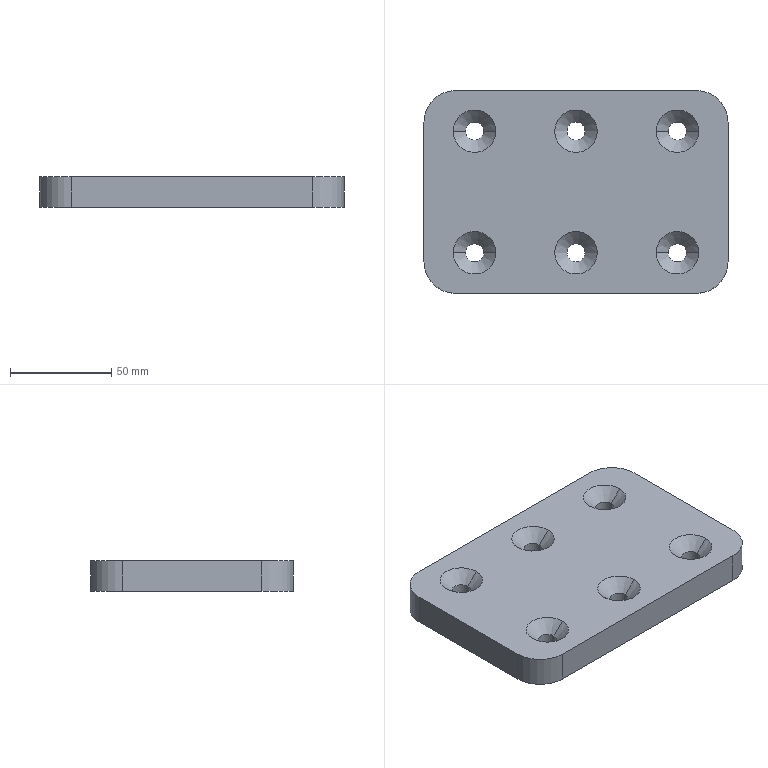Part | SolidWorks | features BaseBody 1 | 1 solid | 48 faces | box 150 x 100 x 15 mm | volume 211756 mm3 | plane 20 | cylinder 16 | cone 12 | commonest cylinder face diameters 9 x12 31 x4
STEP:
#1=CARTESIAN_POINT('',(-50.5,310.,-51.));
#2=VERTEX_POINT('',#1);
#3=CARTESIAN_POINT('',(-41.5,310.,-51.));
#4=VERTEX_POINT('',#3);
#5=CARTESIAN_POINT('',(-46.,310.,-51.));
#6=DIRECTION('',(0.,0.,-1.));
#7=DIRECTION('',(-1.,0.,0.));
#8=AXIS2_PLACEMENT_3D('',#5,#6,#7);
#9=CIRCLE('',#8,4.5);
#10=EDGE_CURVE('',#2,#4,#9,.T.);
#11=ORIENTED_EDGE('',*,*,#10,.F.);
#12=CARTESIAN_POINT('',(-50.5,310.,-60.));
#13=VERTEX_POINT('',#12);
#14=CARTESIAN_POINT('',(-50.5,310.,-40.));
#15=DIRECTION('',(0.,0.,-1.));
#16=VECTOR('',#15,1000.);
#17=LINE('',#14,#16);
#18=EDGE_CURVE('',#2,#13,#17,.T.);
#19=ORIENTED_EDGE('',*,*,#18,.T.);
#20=CARTESIAN_POINT('',(-41.5,310.,-60.));
#21=VERTEX_POINT('',#20);
#22=CARTESIAN_POINT('',(-46.,310.,-60.));
#23=DIRECTION('',(0.,0.,-1.));
#24=DIRECTION('',(1.,0.,0.));
#25=AXIS2_PLACEMENT_3D('',#22,#23,#24);
#26=CIRCLE('',#25,4.5);
#27=EDGE_CURVE('',#13,#21,#26,.T.);
#28=ORIENTED_EDGE('',*,*,#27,.T.);
#29=CARTESIAN_POINT('',(-41.5,310.,-40.));
#30=DIRECTION('',(0.,0.,-1.));
#31=VECTOR('',#30,1000.);
#32=LINE('',#29,#31);
#33=EDGE_CURVE('',#4,#21,#32,.T.);
#34=ORIENTED_EDGE('',*,*,#33,.F.);
#35=EDGE_LOOP('',(#11,#19,#28,#34));
#36=FACE_OUTER_BOUND('',#35,.T.);
#37=CARTESIAN_POINT('',(-46.,310.,-40.));
#38=DIRECTION('',(0.,0.,-1.));
#39=DIRECTION('',(1.,0.,0.));
#40=AXIS2_PLACEMENT_3D('',#37,#38,#39);
#41=CYLINDRICAL_SURFACE('',#40,4.5);
#42=ADVANCED_FACE('',(#36),#41,.F.);
#43=CARTESIAN_POINT('',(-50.5,250.,-51.));
#44=VERTEX_POINT('',#43);
#45=CARTESIAN_POINT('',(-41.5,250.,-51.));
#46=VERTEX_POINT('',#45);
#47=CARTESIAN_POINT('',(-46.,250.,-51.));
#48=DIRECTION('',(0.,0.,-1.));
#49=DIRECTION('',(-1.,0.,0.));
#50=AXIS2_PLACEMENT_3D('',#47,#48,#49);
#51=CIRCLE('',#50,4.5);
#52=EDGE_CURVE('',#44,#46,#51,.T.);
#53=ORIENTED_EDGE('',*,*,#52,.F.);
#54=CARTESIAN_POINT('',(-50.5,250.,-60.));
#55=VERTEX_POINT('',#54);
#56=CARTESIAN_POINT('',(-50.5,250.,-40.));
#57=DIRECTION('',(0.,0.,-1.));
#58=VECTOR('',#57,1000.);
#59=LINE('',#56,#58);
#60=EDGE_CURVE('',#44,#55,#59,.T.);
#61=ORIENTED_EDGE('',*,*,#60,.T.);
#62=CARTESIAN_POINT('',(-41.5,250.,-60.));
#63=VERTEX_POINT('',#62);
#64=CARTESIAN_POINT('',(-46.,250.,-60.));
#65=DIRECTION('',(0.,0.,-1.));
#66=DIRECTION('',(1.,0.,0.));
#67=AXIS2_PLACEMENT_3D('',#64,#65,#66);
#68=CIRCLE('',#67,4.5);
#69=EDGE_CURVE('',#55,#63,#68,.T.);
#70=ORIENTED_EDGE('',*,*,#69,.T.);
#71=CARTESIAN_POINT('',(-41.5,250.,-40.));
#72=DIRECTION('',(0.,0.,-1.));
#73=VECTOR('',#72,1000.);
#74=LINE('',#71,#73);
#75=EDGE_CURVE('',#46,#63,#74,.T.);
#76=ORIENTED_EDGE('',*,*,#75,.F.);
#77=EDGE_LOOP('',(#53,#61,#70,#76));
#78=FACE_OUTER_BOUND('',#77,.T.);
#79=CARTESIAN_POINT('',(-46.,250.,-40.));
#80=DIRECTION('',(0.,0.,-1.));
#81=DIRECTION('',(1.,0.,0.));
#82=AXIS2_PLACEMENT_3D('',#79,#80,#81);
#83=CYLINDRICAL_SURFACE('',#82,4.5);
#84=ADVANCED_FACE('',(#78),#83,.F.);
#85=CARTESIAN_POINT('',(-100.5,310.,-51.));
#86=VERTEX_POINT('',#85);
#87=CARTESIAN_POINT('',(-91.5,310.,-51.));
#88=VERTEX_POINT('',#87);
#89=CARTESIAN_POINT('',(-96.,310.,-51.));
#90=DIRECTION('',(0.,0.,-1.));
#91=DIRECTION('',(-1.,0.,0.));
#92=AXIS2_PLACEMENT_3D('',#89,#90,#91);
#93=CIRCLE('',#92,4.5);
#94=EDGE_CURVE('',#86,#88,#93,.T.);
#95=ORIENTED_EDGE('',*,*,#94,.F.);
#96=CARTESIAN_POINT('',(-100.5,310.,-60.));
#97=VERTEX_POINT('',#96);
#98=CARTESIAN_POINT('',(-100.5,310.,-40.));
#99=DIRECTION('',(0.,0.,-1.));
#100=VECTOR('',#99,1000.);
#101=LINE('',#98,#100);
#102=EDGE_CURVE('',#86,#97,#101,.T.);
#103=ORIENTED_EDGE('',*,*,#102,.T.);
#104=CARTESIAN_POINT('',(-91.5,310.,-60.));
#105=VERTEX_POINT('',#104);
#106=CARTESIAN_POINT('',(-96.,310.,-60.));
#107=DIRECTION('',(0.,0.,-1.));
#108=DIRECTION('',(1.,0.,0.));
#109=AXIS2_PLACEMENT_3D('',#106,#107,#108);
#110=CIRCLE('',#109,4.5);
#111=EDGE_CURVE('',#97,#105,#110,.T.);
#112=ORIENTED_EDGE('',*,*,#111,.T.);
#113=CARTESIAN_POINT('',(-91.5,310.,-40.));
#114=DIRECTION('',(0.,0.,-1.));
#115=VECTOR('',#114,1000.);
#116=LINE('',#113,#115);
#117=EDGE_CURVE('',#88,#105,#116,.T.);
#118=ORIENTED_EDGE('',*,*,#117,.F.);
#119=EDGE_LOOP('',(#95,#103,#112,#118));
#120=FACE_OUTER_BOUND('',#119,.T.);
#121=CARTESIAN_POINT('',(-96.,310.,-40.));
#122=DIRECTION('',(0.,0.,-1.));
#123=DIRECTION('',(1.,0.,0.));
#124=AXIS2_PLACEMENT_3D('',#121,#122,#123);
#125=CYLINDRICAL_SURFACE('',#124,4.5);
#126=ADVANCED_FACE('',(#120),#125,.F.);
#127=CARTESIAN_POINT('',(-150.5,250.,-51.));
#128=VERTEX_POINT('',#127);
#129=CARTESIAN_POINT('',(-141.5,250.,-51.));
#130=VERTEX_POINT('',#129);
#131=CARTESIAN_POINT('',(-146.,250.,-51.));
#132=DIRECTION('',(0.,0.,-1.));
#133=DIRECTION('',(-1.,0.,0.));
#134=AXIS2_PLACEMENT_3D('',#131,#132,#133);
#135=CIRCLE('',#134,4.5);
#136=EDGE_CURVE('',#128,#130,#135,.T.);
#137=ORIENTED_EDGE('',*,*,#136,.F.);
#138=CARTESIAN_POINT('',(-150.5,250.,-60.));
#139=VERTEX_POINT('',#138);
#140=CARTESIAN_POINT('',(-150.5,250.,-40.));
#141=DIRECTION('',(0.,0.,-1.));
#142=VECTOR('',#141,1000.);
#143=LINE('',#140,#142);
#144=EDGE_CURVE('',#128,#139,#143,.T.);
#145=ORIENTED_EDGE('',*,*,#144,.T.);
#146=CARTESIAN_POINT('',(-141.5,250.,-60.));
#147=VERTEX_POINT('',#146);
#148=CARTESIAN_POINT('',(-146.,250.,-60.));
#149=DIRECTION('',(0.,0.,-1.));
#150=DIRECTION('',(1.,0.,0.));
#151=AXIS2_PLACEMENT_3D('',#148,#149,#150);
#152=CIRCLE('',#151,4.5);
#153=EDGE_CURVE('',#139,#147,#152,.T.);
#154=ORIENTED_EDGE('',*,*,#153,.T.);
#155=CARTESIAN_POINT('',(-141.5,250.,-40.));
#156=DIRECTION('',(0.,0.,-1.));
#157=VECTOR('',#156,1000.);
#158=LINE('',#155,#157);
#159=EDGE_CURVE('',#130,#147,#158,.T.);
#160=ORIENTED_EDGE('',*,*,#159,.F.);
#161=EDGE_LOOP('',(#137,#145,#154,#160));
#162=FACE_OUTER_BOUND('',#161,.T.);
#163=CARTESIAN_POINT('',(-146.,250.,-40.));
#164=DIRECTION('',(0.,0.,-1.));
#165=DIRECTION('',(1.,0.,0.));
#166=AXIS2_PLACEMENT_3D('',#163,#164,#165);
#167=CYLINDRICAL_SURFACE('',#166,4.5);
#168=ADVANCED_FACE('',(#162),#167,.F.);
#169=CARTESIAN_POINT('',(-150.5,310.,-51.));
#170=VERTEX_POINT('',#169);
#171=CARTESIAN_POINT('',(-141.5,310.,-51.));
#172=VERTEX_POINT('',#171);
#173=CARTESIAN_POINT('',(-146.,310.,-51.));
#174=DIRECTION('',(0.,0.,-1.));
#175=DIRECTION('',(-1.,0.,0.));
#176=AXIS2_PLACEMENT_3D('',#173,#174,#175);
#177=CIRCLE('',#176,4.5);
#178=EDGE_CURVE('',#170,#172,#177,.T.);
#179=ORIENTED_EDGE('',*,*,#178,.F.);
#180=CARTESIAN_POINT('',(-150.5,310.,-60.));
#181=VERTEX_POINT('',#180);
#182=CARTESIAN_POINT('',(-150.5,310.,-40.));
#183=DIRECTION('',(0.,0.,-1.));
#184=VECTOR('',#183,1000.);
#185=LINE('',#182,#184);
#186=EDGE_CURVE('',#170,#181,#185,.T.);
#187=ORIENTED_EDGE('',*,*,#186,.T.);
#188=CARTESIAN_POINT('',(-141.5,310.,-60.));
#189=VERTEX_POINT('',#188);
#190=CARTESIAN_POINT('',(-146.,310.,-60.));
#191=DIRECTION('',(0.,0.,-1.));
#192=DIRECTION('',(1.,0.,0.));
#193=AXIS2_PLACEMENT_3D('',#190,#191,#192);
#194=CIRCLE('',#193,4.5);
#195=EDGE_CURVE('',#181,#189,#194,.T.);
#196=ORIENTED_EDGE('',*,*,#195,.T.);
#197=CARTESIAN_POINT('',(-141.5,310.,-40.));
#198=DIRECTION('',(0.,0.,-1.));
#199=VECTOR('',#198,1000.);
#200=LINE('',#197,#199);
#201=EDGE_CURVE('',#172,#189,#200,.T.);
#202=ORIENTED_EDGE('',*,*,#201,.F.);
#203=EDGE_LOOP('',(#179,#187,#196,#202));
#204=FACE_OUTER_BOUND('',#203,.T.);
#205=CARTESIAN_POINT('',(-146.,310.,-40.));
#206=DIRECTION('',(0.,0.,-1.));
#207=DIRECTION('',(1.,0.,0.));
#208=AXIS2_PLACEMENT_3D('',#205,#206,#207);
#209=CYLINDRICAL_SURFACE('',#208,4.5);
#210=ADVANCED_FACE('',(#204),#209,.F.);
#211=CARTESIAN_POINT('',(-100.5,250.,-51.));
#212=VERTEX_POINT('',#211);
#213=CARTESIAN_POINT('',(-91.5,250.,-51.));
#214=VERTEX_POINT('',#213);
#215=CARTESIAN_POINT('',(-96.,250.,-51.));
#216=DIRECTION('',(0.,0.,-1.));
#217=DIRECTION('',(-1.,0.,0.));
#218=AXIS2_PLACEMENT_3D('',#215,#216,#217);
#219=CIRCLE('',#218,4.5);
#220=EDGE_CURVE('',#212,#214,#219,.T.);
#221=ORIENTED_EDGE('',*,*,#220,.F.);
#222=CARTESIAN_POINT('',(-100.5,250.,-60.));
#223=VERTEX_POINT('',#222);
#224=CARTESIAN_POINT('',(-100.5,250.,-40.));
#225=DIRECTION('',(0.,0.,-1.));
#226=VECTOR('',#225,1000.);
#227=LINE('',#224,#226);
#228=EDGE_CURVE('',#212,#223,#227,.T.);
#229=ORIENTED_EDGE('',*,*,#228,.T.);
#230=CARTESIAN_POINT('',(-91.5,250.,-60.));
#231=VERTEX_POINT('',#230);
#232=CARTESIAN_POINT('',(-96.,250.,-60.));
#233=DIRECTION('',(0.,0.,-1.));
#234=DIRECTION('',(1.,0.,0.));
#235=AXIS2_PLACEMENT_3D('',#232,#233,#234);
#236=CIRCLE('',#235,4.5);
#237=EDGE_CURVE('',#223,#231,#236,.T.);
#238=ORIENTED_EDGE('',*,*,#237,.T.);
#239=CARTESIAN_POINT('',(-91.5,250.,-40.));
#240=DIRECTION('',(0.,0.,-1.));
#241=VECTOR('',#240,1000.);
#242=LINE('',#239,#241);
#243=EDGE_CURVE('',#214,#231,#242,.T.);
#244=ORIENTED_EDGE('',*,*,#243,.F.);
#245=EDGE_LOOP('',(#221,#229,#238,#244));
#246=FACE_OUTER_BOUND('',#245,.T.);
#247=CARTESIAN_POINT('',(-96.,250.,-40.));
#248=DIRECTION('',(0.,0.,-1.));
#249=DIRECTION('',(1.,0.,0.));
#250=AXIS2_PLACEMENT_3D('',#247,#248,#249);
#251=CYLINDRICAL_SURFACE('',#250,4.5);
#252=ADVANCED_FACE('',(#246),#251,.F.);
#253=CARTESIAN_POINT('',(-46.,310.,-51.));
#254=DIRECTION('',(0.,0.,-1.));
#255=DIRECTION('',(-1.,0.,0.));
#256=AXIS2_PLACEMENT_3D('',#253,#254,#255);
#257=CIRCLE('',#256,4.5);
#258=EDGE_CURVE('',#4,#2,#257,.T.);
#259=ORIENTED_EDGE('',*,*,#258,.T.);
#260=CARTESIAN_POINT('',(-56.5,310.,-45.));
#261=VERTEX_POINT('',#260);
#262=CARTESIAN_POINT('',(-50.5,310.,-51.));
#263=DIRECTION('',(-0.7071,0.,0.7071));
#264=VECTOR('',#263,1000.);
#265=LINE('',#262,#264);
#266=EDGE_CURVE('',#2,#261,#265,.T.);
#267=ORIENTED_EDGE('',*,*,#266,.T.);
#268=CARTESIAN_POINT('',(-35.5,310.,-45.));
#269=VERTEX_POINT('',#268);
#270=CARTESIAN_POINT('',(-46.,310.,-45.));
#271=DIRECTION('',(0.,0.,1.));
#272=DIRECTION('',(-1.,0.,0.));
#273=AXIS2_PLACEMENT_3D('',#270,#271,#272);
#274=CIRCLE('',#273,10.5);
#275=EDGE_CURVE('',#261,#269,#274,.T.);
#276=ORIENTED_EDGE('',*,*,#275,.T.);
#277=CARTESIAN_POINT('',(-41.5,310.,-51.));
#278=DIRECTION('',(0.7071,0.,0.7071));
#279=VECTOR('',#278,1000.);
#280=LINE('',#277,#279);
#281=EDGE_CURVE('',#4,#269,#280,.T.);
#282=ORIENTED_EDGE('',*,*,#281,.F.);
#283=EDGE_LOOP('',(#259,#267,#276,#282));
#284=FACE_OUTER_BOUND('',#283,.T.);
#285=CARTESIAN_POINT('',(-46.,310.,-51.));
#286=DIRECTION('',(0.,0.,1.));
#287=DIRECTION('',(1.,0.,0.));
#288=AXIS2_PLACEMENT_3D('',#285,#286,#287);
#289=CONICAL_SURFACE('',#288,4.5,0.7854);
#290=ADVANCED_FACE('',(#284),#289,.F.);
#291=CARTESIAN_POINT('',(-46.,250.,-51.));
#292=DIRECTION('',(0.,0.,-1.));
#293=DIRECTION('',(-1.,0.,0.));
#294=AXIS2_PLACEMENT_3D('',#291,#292,#293);
#295=CIRCLE('',#294,4.5);
#296=EDGE_CURVE('',#46,#44,#295,.T.);
#297=ORIENTED_EDGE('',*,*,#296,.T.);
#298=CARTESIAN_POINT('',(-56.5,250.,-45.));
#299=VERTEX_POINT('',#298);
#300=CARTESIAN_POINT('',(-50.5,250.,-51.));
#301=DIRECTION('',(-0.7071,0.,0.7071));
#302=VECTOR('',#301,1000.);
#303=LINE('',#300,#302);
#304=EDGE_CURVE('',#44,#299,#303,.T.);
#305=ORIENTED_EDGE('',*,*,#304,.T.);
#306=CARTESIAN_POINT('',(-35.5,250.,-45.));
#307=VERTEX_POINT('',#306);
#308=CARTESIAN_POINT('',(-46.,250.,-45.));
#309=DIRECTION('',(0.,0.,1.));
#310=DIRECTION('',(-1.,0.,0.));
#311=AXIS2_PLACEMENT_3D('',#308,#309,#310);
#312=CIRCLE('',#311,10.5);
#313=EDGE_CURVE('',#299,#307,#312,.T.);
#314=ORIENTED_EDGE('',*,*,#313,.T.);
#315=CARTESIAN_POINT('',(-41.5,250.,-51.));
#316=DIRECTION('',(0.7071,0.,0.7071));
#317=VECTOR('',#316,1000.);
#318=LINE('',#315,#317);
#319=EDGE_CURVE('',#46,#307,#318,.T.);
#320=ORIENTED_EDGE('',*,*,#319,.F.);
#321=EDGE_LOOP('',(#297,#305,#314,#320));
#322=FACE_OUTER_BOUND('',#321,.T.);
#323=CARTESIAN_POINT('',(-46.,250.,-51.));
#324=DIRECTION('',(0.,0.,1.));
#325=DIRECTION('',(1.,0.,0.));
#326=AXIS2_PLACEMENT_3D('',#323,#324,#325);
#327=CONICAL_SURFACE('',#326,4.5,0.7854);
#328=ADVANCED_FACE('',(#322),#327,.F.);
#329=CARTESIAN_POINT('',(-96.,250.,-51.));
#330=DIRECTION('',(0.,0.,-1.));
#331=DIRECTION('',(-1.,0.,0.));
#332=AXIS2_PLACEMENT_3D('',#329,#330,#331);
#333=CIRCLE('',#332,4.5);
#334=EDGE_CURVE('',#214,#212,#333,.T.);
#335=ORIENTED_EDGE('',*,*,#334,.T.);
#336=CARTESIAN_POINT('',(-106.5,250.,-45.));
#337=VERTEX_POINT('',#336);
#338=CARTESIAN_POINT('',(-100.5,250.,-51.));
#339=DIRECTION('',(-0.7071,0.,0.7071));
#340=VECTOR('',#339,1000.);
#341=LINE('',#338,#340);
#342=EDGE_CURVE('',#212,#337,#341,.T.);
#343=ORIENTED_EDGE('',*,*,#342,.T.);
#344=CARTESIAN_POINT('',(-85.5,250.,-45.));
#345=VERTEX_POINT('',#344);
#346=CARTESIAN_POINT('',(-96.,250.,-45.));
#347=DIRECTION('',(0.,0.,1.));
#348=DIRECTION('',(-1.,0.,0.));
#349=AXIS2_PLACEMENT_3D('',#346,#347,#348);
#350=CIRCLE('',#349,10.5);
#351=EDGE_CURVE('',#337,#345,#350,.T.);
#352=ORIENTED_EDGE('',*,*,#351,.T.);
#353=CARTESIAN_POINT('',(-91.5,250.,-51.));
#354=DIRECTION('',(0.7071,0.,0.7071));
#355=VECTOR('',#354,1000.);
#356=LINE('',#353,#355);
#357=EDGE_CURVE('',#214,#345,#356,.T.);
#358=ORIENTED_EDGE('',*,*,#357,.F.);
#359=EDGE_LOOP('',(#335,#343,#352,#358));
#360=FACE_OUTER_BOUND('',#359,.T.);
#361=CARTESIAN_POINT('',(-96.,250.,-51.));
#362=DIRECTION('',(0.,0.,1.));
#363=DIRECTION('',(1.,0.,0.));
#364=AXIS2_PLACEMENT_3D('',#361,#362,#363);
#365=CONICAL_SURFACE('',#364,4.5,0.7854);
#366=ADVANCED_FACE('',(#360),#365,.F.);
#367=CARTESIAN_POINT('',(-96.,310.,-51.));
#368=DIRECTION('',(0.,0.,-1.));
#369=DIRECTION('',(-1.,0.,0.));
#370=AXIS2_PLACEMENT_3D('',#367,#368,#369);
#371=CIRCLE('',#370,4.5);
#372=EDGE_CURVE('',#88,#86,#371,.T.);
#373=ORIENTED_EDGE('',*,*,#372,.T.);
#374=CARTESIAN_POINT('',(-106.5,310.,-45.));
#375=VERTEX_POINT('',#374);
#376=CARTESIAN_POINT('',(-100.5,310.,-51.));
#377=DIRECTION('',(-0.7071,0.,0.7071));
#378=VECTOR('',#377,1000.);
#379=LINE('',#376,#378);
#380=EDGE_CURVE('',#86,#375,#379,.T.);
#381=ORIENTED_EDGE('',*,*,#380,.T.);
#382=CARTESIAN_POINT('',(-85.5,310.,-45.));
#383=VERTEX_POINT('',#382);
#384=CARTESIAN_POINT('',(-96.,310.,-45.));
#385=DIRECTION('',(0.,0.,1.));
#386=DIRECTION('',(-1.,0.,0.));
#387=AXIS2_PLACEMENT_3D('',#384,#385,#386);
#388=CIRCLE('',#387,10.5);
#389=EDGE_CURVE('',#375,#383,#388,.T.);
#390=ORIENTED_EDGE('',*,*,#389,.T.);
#391=CARTESIAN_POINT('',(-91.5,310.,-51.));
#392=DIRECTION('',(0.7071,0.,0.7071));
#393=VECTOR('',#392,1000.);
#394=LINE('',#391,#393);
#395=EDGE_CURVE('',#88,#383,#394,.T.);
#396=ORIENTED_EDGE('',*,*,#395,.F.);
#397=EDGE_LOOP('',(#373,#381,#390,#396));
#398=FACE_OUTER_BOUND('',#397,.T.);
#399=CARTESIAN_POINT('',(-96.,310.,-51.));
#400=DIRECTION('',(0.,0.,1.));
#401=DIRECTION('',(1.,0.,0.));
#402=AXIS2_PLACEMENT_3D('',#399,#400,#401);
#403=CONICAL_SURFACE('',#402,4.5,0.7854);
#404=ADVANCED_FACE('',(#398),#403,.F.);
#405=CARTESIAN_POINT('',(-146.,310.,-51.));
#406=DIRECTION('',(0.,0.,-1.));
#407=DIRECTION('',(-1.,0.,0.));
#408=AXIS2_PLACEMENT_3D('',#405,#406,#407);
#409=CIRCLE('',#408,4.5);
#410=EDGE_CURVE('',#172,#170,#409,.T.);
#411=ORIENTED_EDGE('',*,*,#410,.T.);
#412=CARTESIAN_POINT('',(-156.5,310.,-45.));
#413=VERTEX_POINT('',#412);
#414=CARTESIAN_POINT('',(-150.5,310.,-51.));
#415=DIRECTION('',(-0.7071,0.,0.7071));
#416=VECTOR('',#415,1000.);
#417=LINE('',#414,#416);
#418=EDGE_CURVE('',#170,#413,#417,.T.);
#419=ORIENTED_EDGE('',*,*,#418,.T.);
#420=CARTESIAN_POINT('',(-135.5,310.,-45.));
#421=VERTEX_POINT('',#420);
#422=CARTESIAN_POINT('',(-146.,310.,-45.));
#423=DIRECTION('',(0.,0.,1.));
#424=DIRECTION('',(-1.,0.,0.));
#425=AXIS2_PLACEMENT_3D('',#422,#423,#424);
#426=CIRCLE('',#425,10.5);
#427=EDGE_CURVE('',#413,#421,#426,.T.);
#428=ORIENTED_EDGE('',*,*,#427,.T.);
#429=CARTESIAN_POINT('',(-141.5,310.,-51.));
#430=DIRECTION('',(0.7071,0.,0.7071));
#431=VECTOR('',#430,1000.);
#432=LINE('',#429,#431);
#433=EDGE_CURVE('',#172,#421,#432,.T.);
#434=ORIENTED_EDGE('',*,*,#433,.F.);
#435=EDGE_LOOP('',(#411,#419,#428,#434));
#436=FACE_OUTER_BOUND('',#435,.T.);
#437=CARTESIAN_POINT('',(-146.,310.,-51.));
#438=DIRECTION('',(0.,0.,1.));
#439=DIRECTION('',(1.,0.,0.));
#440=AXIS2_PLACEMENT_3D('',#437,#438,#439);
#441=CONICAL_SURFACE('',#440,4.5,0.7854);
#442=ADVANCED_FACE('',(#436),#441,.F.);
#443=CARTESIAN_POINT('',(-146.,250.,-51.));
#444=DIRECTION('',(0.,0.,-1.));
#445=DIRECTION('',(-1.,0.,0.));
#446=AXIS2_PLACEMENT_3D('',#443,#444,#445);
#447=CIRCLE('',#446,4.5);
#448=EDGE_CURVE('',#130,#128,#447,.T.);
#449=ORIENTED_EDGE('',*,*,#448,.T.);
#450=CARTESIAN_POINT('',(-156.5,250.,-45.));
#451=VERTEX_POINT('',#450);
#452=CARTESIAN_POINT('',(-150.5,250.,-51.));
#453=DIRECTION('',(-0.7071,0.,0.7071));
#454=VECTOR('',#453,1000.);
#455=LINE('',#452,#454);
#456=EDGE_CURVE('',#128,#451,#455,.T.);
#457=ORIENTED_EDGE('',*,*,#456,.T.);
#458=CARTESIAN_POINT('',(-135.5,250.,-45.));
#459=VERTEX_POINT('',#458);
#460=CARTESIAN_POINT('',(-146.,250.,-45.));
#461=DIRECTION('',(0.,0.,1.));
#462=DIRECTION('',(-1.,0.,0.));
#463=AXIS2_PLACEMENT_3D('',#460,#461,#462);
#464=CIRCLE('',#463,10.5);
#465=EDGE_CURVE('',#451,#459,#464,.T.);
#466=ORIENTED_EDGE('',*,*,#465,.T.);
#467=CARTESIAN_POINT('',(-141.5,250.,-51.));
#468=DIRECTION('',(0.7071,0.,0.7071));
#469=VECTOR('',#468,1000.);
#470=LINE('',#467,#469);
#471=EDGE_CURVE('',#130,#459,#470,.T.);
#472=ORIENTED_EDGE('',*,*,#471,.F.);
#473=EDGE_LOOP('',(#449,#457,#466,#472));
#474=FACE_OUTER_BOUND('',#473,.T.);
#475=CARTESIAN_POINT('',(-146.,250.,-51.));
#476=DIRECTION('',(0.,0.,1.));
#477=DIRECTION('',(1.,0.,0.));
#478=AXIS2_PLACEMENT_3D('',#475,#476,#477);
#479=CONICAL_SURFACE('',#478,4.5,0.7854);
#480=ADVANCED_FACE('',(#474),#479,.F.);
#481=CARTESIAN_POINT('',(-46.,250.,-60.));
#482=DIRECTION('',(0.,0.,-1.));
#483=DIRECTION('',(1.,0.,0.));
#484=AXIS2_PLACEMENT_3D('',#481,#482,#483);
#485=CIRCLE('',#484,4.5);
#486=EDGE_CURVE('',#63,#55,#485,.T.);
#487=ORIENTED_EDGE('',*,*,#486,.F.);
#488=ORIENTED_EDGE('',*,*,#69,.F.);
#489=EDGE_LOOP('',(#487,#488));
#490=FACE_BOUND('',#489,.T.);
#491=CARTESIAN_POINT('',(-96.,310.,-60.));
#492=DIRECTION('',(0.,0.,-1.));
#493=DIRECTION('',(1.,0.,0.));
#494=AXIS2_PLACEMENT_3D('',#491,#492,#493);
#495=CIRCLE('',#494,4.5);
#496=EDGE_CURVE('',#105,#97,#495,.T.);
#497=ORIENTED_EDGE('',*,*,#496,.F.);
#498=ORIENTED_EDGE('',*,*,#111,.F.);
#499=EDGE_LOOP('',(#497,#498));
#500=FACE_BOUND('',#499,.T.);
#501=CARTESIAN_POINT('',(-146.,250.,-60.));
#502=DIRECTION('',(0.,0.,-1.));
#503=DIRECTION('',(1.,0.,0.));
#504=AXIS2_PLACEMENT_3D('',#501,#502,#503);
#505=CIRCLE('',#504,4.5);
#506=EDGE_CURVE('',#147,#139,#505,.T.);
#507=ORIENTED_EDGE('',*,*,#506,.F.);
#508=ORIENTED_EDGE('',*,*,#153,.F.);
#509=EDGE_LOOP('',(#507,#508));
#510=FACE_BOUND('',#509,.T.);
#511=CARTESIAN_POINT('',(-21.,314.5,-60.));
#512=VERTEX_POINT('',#511);
#513=CARTESIAN_POINT('',(-21.,245.5,-60.));
#514=VERTEX_POINT('',#513);
#515=CARTESIAN_POINT('',(-21.,280.,-60.));
#516=DIRECTION('',(0.,-1.,0.));
#517=VECTOR('',#516,1000.);
#518=LINE('',#515,#517);
#519=EDGE_CURVE('',#512,#514,#518,.T.);
#520=ORIENTED_EDGE('',*,*,#519,.T.);
#521=CARTESIAN_POINT('',(-36.5,230.,-60.));
#522=VERTEX_POINT('',#521);
#523=CARTESIAN_POINT('',(-36.5,245.5,-60.));
#524=DIRECTION('',(0.,0.,1.));
#525=DIRECTION('',(1.,0.,0.));
#526=AXIS2_PLACEMENT_3D('',#523,#524,#525);
#527=CIRCLE('',#526,15.5);
#528=EDGE_CURVE('',#522,#514,#527,.T.);
#529=ORIENTED_EDGE('',*,*,#528,.F.);
#530=CARTESIAN_POINT('',(-155.5,230.,-60.));
#531=VERTEX_POINT('',#530);
#532=CARTESIAN_POINT('',(0.,230.,-60.));
#533=DIRECTION('',(-1.,0.,0.));
#534=VECTOR('',#533,1000.);
#535=LINE('',#532,#534);
#536=EDGE_CURVE('',#522,#531,#535,.T.);
#537=ORIENTED_EDGE('',*,*,#536,.T.);
#538=CARTESIAN_POINT('',(-171.,245.5,-60.));
#539=VERTEX_POINT('',#538);
#540=CARTESIAN_POINT('',(-155.5,245.5,-60.));
#541=DIRECTION('',(0.,0.,1.));
#542=DIRECTION('',(1.,0.,0.));
#543=AXIS2_PLACEMENT_3D('',#540,#541,#542);
#544=CIRCLE('',#543,15.5);
#545=EDGE_CURVE('',#539,#531,#544,.T.);
#546=ORIENTED_EDGE('',*,*,#545,.F.);
#547=CARTESIAN_POINT('',(-171.,314.5,-60.));
#548=VERTEX_POINT('',#547);
#549=CARTESIAN_POINT('',(-171.,280.,-60.));
#550=DIRECTION('',(0.,1.,0.));
#551=VECTOR('',#550,1000.);
#552=LINE('',#549,#551);
#553=EDGE_CURVE('',#539,#548,#552,.T.);
#554=ORIENTED_EDGE('',*,*,#553,.T.);
#555=CARTESIAN_POINT('',(-155.5,330.,-60.));
#556=VERTEX_POINT('',#555);
#557=CARTESIAN_POINT('',(-155.5,314.5,-60.));
#558=DIRECTION('',(0.,0.,1.));
#559=DIRECTION('',(1.,0.,0.));
#560=AXIS2_PLACEMENT_3D('',#557,#558,#559);
#561=CIRCLE('',#560,15.5);
#562=EDGE_CURVE('',#556,#548,#561,.T.);
#563=ORIENTED_EDGE('',*,*,#562,.F.);
#564=CARTESIAN_POINT('',(-36.5,330.,-60.));
#565=VERTEX_POINT('',#564);
#566=CARTESIAN_POINT('',(0.,330.,-60.));
#567=DIRECTION('',(1.,0.,0.));
#568=VECTOR('',#567,1000.);
#569=LINE('',#566,#568);
#570=EDGE_CURVE('',#556,#565,#569,.T.);
#571=ORIENTED_EDGE('',*,*,#570,.T.);
#572=CARTESIAN_POINT('',(-36.5,314.5,-60.));
#573=DIRECTION('',(0.,0.,1.));
#574=DIRECTION('',(1.,0.,0.));
#575=AXIS2_PLACEMENT_3D('',#572,#573,#574);
#576=CIRCLE('',#575,15.5);
#577=EDGE_CURVE('',#512,#565,#576,.T.);
#578=ORIENTED_EDGE('',*,*,#577,.F.);
#579=EDGE_LOOP('',(#520,#529,#537,#546,#554,#563,#571,#578));
#580=FACE_OUTER_BOUND('',#579,.T.);
#581=CARTESIAN_POINT('',(-146.,310.,-60.));
#582=DIRECTION('',(0.,0.,-1.));
#583=DIRECTION('',(1.,0.,0.));
#584=AXIS2_PLACEMENT_3D('',#581,#582,#583);
#585=CIRCLE('',#584,4.5);
#586=EDGE_CURVE('',#189,#181,#585,.T.);
#587=ORIENTED_EDGE('',*,*,#586,.F.);
#588=ORIENTED_EDGE('',*,*,#195,.F.);
#589=EDGE_LOOP('',(#587,#588));
#590=FACE_BOUND('',#589,.T.);
#591=CARTESIAN_POINT('',(-96.,250.,-60.));
#592=DIRECTION('',(0.,0.,-1.));
#593=DIRECTION('',(1.,0.,0.));
#594=AXIS2_PLACEMENT_3D('',#591,#592,#593);
#595=CIRCLE('',#594,4.5);
#596=EDGE_CURVE('',#231,#223,#595,.T.);
#597=ORIENTED_EDGE('',*,*,#596,.F.);
#598=ORIENTED_EDGE('',*,*,#237,.F.);
#599=EDGE_LOOP('',(#597,#598));
#600=FACE_BOUND('',#599,.T.);
#601=CARTESIAN_POINT('',(-46.,310.,-60.));
#602=DIRECTION('',(0.,0.,-1.));
#603=DIRECTION('',(1.,0.,0.));
#604=AXIS2_PLACEMENT_3D('',#601,#602,#603);
#605=CIRCLE('',#604,4.5);
#606=EDGE_CURVE('',#21,#13,#605,.T.);
#607=ORIENTED_EDGE('',*,*,#606,.F.);
#608=ORIENTED_EDGE('',*,*,#27,.F.);
#609=EDGE_LOOP('',(#607,#608));
#610=FACE_BOUND('',#609,.T.);
#611=CARTESIAN_POINT('',(-159.947,314.357,-60.));
#612=VERTEX_POINT('',#611);
#613=CARTESIAN_POINT('',(-159.947,310.357,-60.));
#614=VERTEX_POINT('',#613);
#615=CARTESIAN_POINT('',(-159.947,314.357,-60.));
#616=DIRECTION('',(0.,-1.,0.));
#617=VECTOR('',#616,1000.);
#618=LINE('',#615,#617);
#619=EDGE_CURVE('',#612,#614,#618,.T.);
#620=ORIENTED_EDGE('',*,*,#619,.F.);
#621=CARTESIAN_POINT('',(-154.947,314.357,-60.));
#622=VERTEX_POINT('',#621);
#623=CARTESIAN_POINT('',(-159.947,314.357,-60.));
#624=DIRECTION('',(1.,0.,0.));
#625=VECTOR('',#624,1000.);
#626=LINE('',#623,#625);
#627=EDGE_CURVE('',#612,#622,#626,.T.);
#628=ORIENTED_EDGE('',*,*,#627,.T.);
#629=CARTESIAN_POINT('',(-154.947,319.357,-60.));
#630=VERTEX_POINT('',#629);
#631=CARTESIAN_POINT('',(-154.947,319.357,-60.));
#632=DIRECTION('',(0.,-1.,0.));
#633=VECTOR('',#632,1000.);
#634=LINE('',#631,#633);
#635=EDGE_CURVE('',#630,#622,#634,.T.);
#636=ORIENTED_EDGE('',*,*,#635,.F.);
#637=CARTESIAN_POINT('',(-150.947,319.357,-60.));
#638=VERTEX_POINT('',#637);
#639=CARTESIAN_POINT('',(-154.947,319.357,-60.));
#640=DIRECTION('',(1.,0.,0.));
#641=VECTOR('',#640,1000.);
#642=LINE('',#639,#641);
#643=EDGE_CURVE('',#630,#638,#642,.T.);
#644=ORIENTED_EDGE('',*,*,#643,.T.);
#645=CARTESIAN_POINT('',(-150.947,320.357,-60.));
#646=VERTEX_POINT('',#645);
#647=CARTESIAN_POINT('',(-150.947,319.357,-60.));
#648=DIRECTION('',(0.,1.,0.));
#649=VECTOR('',#648,1000.);
#650=LINE('',#647,#649);
#651=EDGE_CURVE('',#638,#646,#650,.T.);
#652=ORIENTED_EDGE('',*,*,#651,.T.);
#653=CARTESIAN_POINT('',(-160.947,320.357,-60.));
#654=VERTEX_POINT('',#653);
#655=CARTESIAN_POINT('',(-160.947,320.357,-60.));
#656=DIRECTION('',(1.,0.,0.));
#657=VECTOR('',#656,1000.);
#658=LINE('',#655,#657);
#659=EDGE_CURVE('',#654,#646,#658,.T.);
#660=ORIENTED_EDGE('',*,*,#659,.F.);
#661=CARTESIAN_POINT('',(-160.947,310.357,-60.));
#662=VERTEX_POINT('',#661);
#663=CARTESIAN_POINT('',(-160.947,320.357,-60.));
#664=DIRECTION('',(0.,-1.,0.));
#665=VECTOR('',#664,1000.);
#666=LINE('',#663,#665);
#667=EDGE_CURVE('',#654,#662,#666,.T.);
#668=ORIENTED_EDGE('',*,*,#667,.T.);
#669=CARTESIAN_POINT('',(-160.947,310.357,-60.));
#670=DIRECTION('',(1.,0.,0.));
#671=VECTOR('',#670,1000.);
#672=LINE('',#669,#671);
#673=EDGE_CURVE('',#662,#614,#672,.T.);
#674=ORIENTED_EDGE('',*,*,#673,.T.);
#675=EDGE_LOOP('',(#620,#628,#636,#644,#652,#660,#668,#674));
#676=FACE_BOUND('',#675,.T.);
#677=CARTESIAN_POINT('',(0.,280.,-60.));
#678=DIRECTION('',(0.,0.,-1.));
#679=DIRECTION('',(1.,0.,0.));
#680=AXIS2_PLACEMENT_3D('',#677,#678,#679);
#681=PLANE('',#680);
#682=ADVANCED_FACE('',(#490,#500,#510,#580,#590,#600,#610,#676),#681,.T.);
#683=CARTESIAN_POINT('',(-46.,250.,-45.));
#684=DIRECTION('',(0.,0.,1.));
#685=DIRECTION('',(-1.,0.,0.));
#686=AXIS2_PLACEMENT_3D('',#683,#684,#685);
#687=CIRCLE('',#686,10.5);
#688=EDGE_CURVE('',#307,#299,#687,.T.);
#689=ORIENTED_EDGE('',*,*,#688,.F.);
#690=ORIENTED_EDGE('',*,*,#313,.F.);
#691=EDGE_LOOP('',(#689,#690));
#692=FACE_BOUND('',#691,.T.);
#693=CARTESIAN_POINT('',(-96.,310.,-45.));
#694=DIRECTION('',(0.,0.,1.));
#695=DIRECTION('',(-1.,0.,0.));
#696=AXIS2_PLACEMENT_3D('',#693,#694,#695);
#697=CIRCLE('',#696,10.5);
#698=EDGE_CURVE('',#383,#375,#697,.T.);
#699=ORIENTED_EDGE('',*,*,#698,.F.);
#700=ORIENTED_EDGE('',*,*,#389,.F.);
#701=EDGE_LOOP('',(#699,#700));
#702=FACE_BOUND('',#701,.T.);
#703=CARTESIAN_POINT('',(-146.,250.,-45.));
#704=DIRECTION('',(0.,0.,1.));
#705=DIRECTION('',(-1.,0.,0.));
#706=AXIS2_PLACEMENT_3D('',#703,#704,#705);
#707=CIRCLE('',#706,10.5);
#708=EDGE_CURVE('',#459,#451,#707,.T.);
#709=ORIENTED_EDGE('',*,*,#708,.F.);
#710=ORIENTED_EDGE('',*,*,#465,.F.);
#711=EDGE_LOOP('',(#709,#710));
#712=FACE_BOUND('',#711,.T.);
#713=CARTESIAN_POINT('',(-36.5,330.,-45.));
#714=VERTEX_POINT('',#713);
#715=CARTESIAN_POINT('',(-155.5,330.,-45.));
#716=VERTEX_POINT('',#715);
#717=CARTESIAN_POINT('',(0.,330.,-45.));
#718=DIRECTION('',(-1.,0.,0.));
#719=VECTOR('',#718,1000.);
#720=LINE('',#717,#719);
#721=EDGE_CURVE('',#714,#716,#720,.T.);
#722=ORIENTED_EDGE('',*,*,#721,.T.);
#723=CARTESIAN_POINT('',(-171.,314.5,-45.));
#724=VERTEX_POINT('',#723);
#725=CARTESIAN_POINT('',(-155.5,314.5,-45.));
#726=DIRECTION('',(0.,0.,-1.));
#727=DIRECTION('',(-1.,0.,0.));
#728=AXIS2_PLACEMENT_3D('',#725,#726,#727);
#729=CIRCLE('',#728,15.5);
#730=EDGE_CURVE('',#724,#716,#729,.T.);
#731=ORIENTED_EDGE('',*,*,#730,.F.);
#732=CARTESIAN_POINT('',(-171.,245.5,-45.));
#733=VERTEX_POINT('',#732);
#734=CARTESIAN_POINT('',(-171.,280.,-45.));
#735=DIRECTION('',(0.,-1.,0.));
#736=VECTOR('',#735,1000.);
#737=LINE('',#734,#736);
#738=EDGE_CURVE('',#724,#733,#737,.T.);
#739=ORIENTED_EDGE('',*,*,#738,.T.);
#740=CARTESIAN_POINT('',(-155.5,230.,-45.));
#741=VERTEX_POINT('',#740);
#742=CARTESIAN_POINT('',(-155.5,245.5,-45.));
#743=DIRECTION('',(0.,0.,-1.));
#744=DIRECTION('',(-1.,0.,0.));
#745=AXIS2_PLACEMENT_3D('',#742,#743,#744);
#746=CIRCLE('',#745,15.5);
#747=EDGE_CURVE('',#741,#733,#746,.T.);
#748=ORIENTED_EDGE('',*,*,#747,.F.);
#749=CARTESIAN_POINT('',(-36.5,230.,-45.));
#750=VERTEX_POINT('',#749);
#751=CARTESIAN_POINT('',(0.,230.,-45.));
#752=DIRECTION('',(1.,0.,0.));
#753=VECTOR('',#752,1000.);
#754=LINE('',#751,#753);
#755=EDGE_CURVE('',#741,#750,#754,.T.);
#756=ORIENTED_EDGE('',*,*,#755,.T.);
#757=CARTESIAN_POINT('',(-21.,245.5,-45.));
#758=VERTEX_POINT('',#757);
#759=CARTESIAN_POINT('',(-36.5,245.5,-45.));
#760=DIRECTION('',(0.,0.,-1.));
#761=DIRECTION('',(-1.,0.,0.));
#762=AXIS2_PLACEMENT_3D('',#759,#760,#761);
#763=CIRCLE('',#762,15.5);
#764=EDGE_CURVE('',#758,#750,#763,.T.);
#765=ORIENTED_EDGE('',*,*,#764,.F.);
#766=CARTESIAN_POINT('',(-21.,314.5,-45.));
#767=VERTEX_POINT('',#766);
#768=CARTESIAN_POINT('',(-21.,280.,-45.));
#769=DIRECTION('',(0.,1.,0.));
#770=VECTOR('',#769,1000.);
#771=LINE('',#768,#770);
#772=EDGE_CURVE('',#758,#767,#771,.T.);
#773=ORIENTED_EDGE('',*,*,#772,.T.);
#774=CARTESIAN_POINT('',(-36.5,314.5,-45.));
#775=DIRECTION('',(0.,0.,-1.));
#776=DIRECTION('',(-1.,0.,0.));
#777=AXIS2_PLACEMENT_3D('',#774,#775,#776);
#778=CIRCLE('',#777,15.5);
#779=EDGE_CURVE('',#714,#767,#778,.T.);
#780=ORIENTED_EDGE('',*,*,#779,.F.);
#781=EDGE_LOOP('',(#722,#731,#739,#748,#756,#765,#773,#780));
#782=FACE_OUTER_BOUND('',#781,.T.);
#783=CARTESIAN_POINT('',(-146.,310.,-45.));
#784=DIRECTION('',(0.,0.,1.));
#785=DIRECTION('',(-1.,0.,0.));
#786=AXIS2_PLACEMENT_3D('',#783,#784,#785);
#787=CIRCLE('',#786,10.5);
#788=EDGE_CURVE('',#421,#413,#787,.T.);
#789=ORIENTED_EDGE('',*,*,#788,.F.);
#790=ORIENTED_EDGE('',*,*,#427,.F.);
#791=EDGE_LOOP('',(#789,#790));
#792=FACE_BOUND('',#791,.T.);
#793=CARTESIAN_POINT('',(-96.,250.,-45.));
#794=DIRECTION('',(0.,0.,1.));
#795=DIRECTION('',(-1.,0.,0.));
#796=AXIS2_PLACEMENT_3D('',#793,#794,#795);
#797=CIRCLE('',#796,10.5);
#798=EDGE_CURVE('',#345,#337,#797,.T.);
#799=ORIENTED_EDGE('',*,*,#798,.F.);
#800=ORIENTED_EDGE('',*,*,#351,.F.);
#801=EDGE_LOOP('',(#799,#800));
#802=FACE_BOUND('',#801,.T.);
#803=CARTESIAN_POINT('',(-46.,310.,-45.));
#804=DIRECTION('',(0.,0.,1.));
#805=DIRECTION('',(-1.,0.,0.));
#806=AXIS2_PLACEMENT_3D('',#803,#804,#805);
#807=CIRCLE('',#806,10.5);
#808=EDGE_CURVE('',#269,#261,#807,.T.);
#809=ORIENTED_EDGE('',*,*,#808,.F.);
#810=ORIENTED_EDGE('',*,*,#275,.F.);
#811=EDGE_LOOP('',(#809,#810));
#812=FACE_BOUND('',#811,.T.);
#813=CARTESIAN_POINT('',(0.,280.,-45.));
#814=DIRECTION('',(0.,0.,1.));
#815=DIRECTION('',(-1.,0.,0.));
#816=AXIS2_PLACEMENT_3D('',#813,#814,#815);
#817=PLANE('',#816);
#818=ADVANCED_FACE('',(#692,#702,#712,#782,#792,#802,#812),#817,.T.);
#819=CARTESIAN_POINT('',(-36.5,230.,-60.));
#820=DIRECTION('',(0.,0.,-1.));
#821=VECTOR('',#820,1000.);
#822=LINE('',#819,#821);
#823=EDGE_CURVE('',#750,#522,#822,.T.);
#824=ORIENTED_EDGE('',*,*,#823,.F.);
#825=ORIENTED_EDGE('',*,*,#755,.F.);
#826=CARTESIAN_POINT('',(-155.5,230.,-60.));
#827=DIRECTION('',(0.,0.,1.));
#828=VECTOR('',#827,1000.);
#829=LINE('',#826,#828);
#830=EDGE_CURVE('',#531,#741,#829,.T.);
#831=ORIENTED_EDGE('',*,*,#830,.F.);
#832=ORIENTED_EDGE('',*,*,#536,.F.);
#833=EDGE_LOOP('',(#824,#825,#831,#832));
#834=FACE_OUTER_BOUND('',#833,.T.);
#835=CARTESIAN_POINT('',(0.,230.,-60.));
#836=DIRECTION('',(0.,-1.,0.));
#837=DIRECTION('',(0.,0.,-1.));
#838=AXIS2_PLACEMENT_3D('',#835,#836,#837);
#839=PLANE('',#838);
#840=ADVANCED_FACE('',(#834),#839,.T.);
#841=CARTESIAN_POINT('',(-155.5,330.,-60.));
#842=DIRECTION('',(0.,0.,-1.));
#843=VECTOR('',#842,1000.);
#844=LINE('',#841,#843);
#845=EDGE_CURVE('',#716,#556,#844,.T.);
#846=ORIENTED_EDGE('',*,*,#845,.F.);
#847=ORIENTED_EDGE('',*,*,#721,.F.);
#848=CARTESIAN_POINT('',(-36.5,330.,-45.));
#849=DIRECTION('',(0.,0.,1.));
#850=VECTOR('',#849,1000.);
#851=LINE('',#848,#850);
#852=EDGE_CURVE('',#565,#714,#851,.T.);
#853=ORIENTED_EDGE('',*,*,#852,.F.);
#854=ORIENTED_EDGE('',*,*,#570,.F.);
#855=EDGE_LOOP('',(#846,#847,#853,#854));
#856=FACE_OUTER_BOUND('',#855,.T.);
#857=CARTESIAN_POINT('',(0.,330.,-60.));
#858=DIRECTION('',(0.,1.,0.));
#859=DIRECTION('',(0.,0.,1.));
#860=AXIS2_PLACEMENT_3D('',#857,#858,#859);
#861=PLANE('',#860);
#862=ADVANCED_FACE('',(#856),#861,.T.);
#863=CARTESIAN_POINT('',(-171.,245.5,-60.));
#864=DIRECTION('',(0.,0.,-1.));
#865=VECTOR('',#864,1000.);
#866=LINE('',#863,#865);
#867=EDGE_CURVE('',#733,#539,#866,.T.);
#868=ORIENTED_EDGE('',*,*,#867,.F.);
#869=ORIENTED_EDGE('',*,*,#738,.F.);
#870=CARTESIAN_POINT('',(-171.,314.5,-60.));
#871=DIRECTION('',(0.,0.,1.));
#872=VECTOR('',#871,1000.);
#873=LINE('',#870,#872);
#874=EDGE_CURVE('',#548,#724,#873,.T.);
#875=ORIENTED_EDGE('',*,*,#874,.F.);
#876=ORIENTED_EDGE('',*,*,#553,.F.);
#877=EDGE_LOOP('',(#868,#869,#875,#876));
#878=FACE_OUTER_BOUND('',#877,.T.);
#879=CARTESIAN_POINT('',(-171.,280.,-60.));
#880=DIRECTION('',(-1.,0.,0.));
#881=DIRECTION('',(0.,0.,-1.));
#882=AXIS2_PLACEMENT_3D('',#879,#880,#881);
#883=PLANE('',#882);
#884=ADVANCED_FACE('',(#878),#883,.T.);
#885=CARTESIAN_POINT('',(-21.,314.5,-60.));
#886=DIRECTION('',(0.,0.,-1.));
#887=VECTOR('',#886,1000.);
#888=LINE('',#885,#887);
#889=EDGE_CURVE('',#767,#512,#888,.T.);
#890=ORIENTED_EDGE('',*,*,#889,.F.);
#891=ORIENTED_EDGE('',*,*,#772,.F.);
#892=CARTESIAN_POINT('',(-21.,245.5,-45.));
#893=DIRECTION('',(0.,0.,1.));
#894=VECTOR('',#893,1000.);
#895=LINE('',#892,#894);
#896=EDGE_CURVE('',#514,#758,#895,.T.);
#897=ORIENTED_EDGE('',*,*,#896,.F.);
#898=ORIENTED_EDGE('',*,*,#519,.F.);
#899=EDGE_LOOP('',(#890,#891,#897,#898));
#900=FACE_OUTER_BOUND('',#899,.T.);
#901=CARTESIAN_POINT('',(-21.,330.,-45.));
#902=DIRECTION('',(-1.,0.,0.));
#903=DIRECTION('',(0.,0.,-1.));
#904=AXIS2_PLACEMENT_3D('',#901,#902,#903);
#905=PLANE('',#904);
#906=ADVANCED_FACE('',(#900),#905,.F.);
#907=ORIENTED_EDGE('',*,*,#852,.T.);
#908=ORIENTED_EDGE('',*,*,#779,.T.);
#909=ORIENTED_EDGE('',*,*,#889,.T.);
#910=ORIENTED_EDGE('',*,*,#577,.T.);
#911=EDGE_LOOP('',(#907,#908,#909,#910));
#912=FACE_OUTER_BOUND('',#911,.T.);
#913=CARTESIAN_POINT('',(-36.5,314.5,-45.));
#914=DIRECTION('',(0.,0.,1.));
#915=DIRECTION('',(-1.,0.,0.));
#916=AXIS2_PLACEMENT_3D('',#913,#914,#915);
#917=CYLINDRICAL_SURFACE('',#916,15.5);
#918=ADVANCED_FACE('',(#912),#917,.T.);
#919=ORIENTED_EDGE('',*,*,#896,.T.);
#920=ORIENTED_EDGE('',*,*,#764,.T.);
#921=ORIENTED_EDGE('',*,*,#823,.T.);
#922=ORIENTED_EDGE('',*,*,#528,.T.);
#923=EDGE_LOOP('',(#919,#920,#921,#922));
#924=FACE_OUTER_BOUND('',#923,.T.);
#925=CARTESIAN_POINT('',(-36.5,245.5,-45.));
#926=DIRECTION('',(0.,0.,-1.));
#927=DIRECTION('',(1.,0.,0.));
#928=AXIS2_PLACEMENT_3D('',#925,#926,#927);
#929=CYLINDRICAL_SURFACE('',#928,15.5);
#930=ADVANCED_FACE('',(#924),#929,.T.);
#931=ORIENTED_EDGE('',*,*,#874,.T.);
#932=ORIENTED_EDGE('',*,*,#730,.T.);
#933=ORIENTED_EDGE('',*,*,#845,.T.);
#934=ORIENTED_EDGE('',*,*,#562,.T.);
#935=EDGE_LOOP('',(#931,#932,#933,#934));
#936=FACE_OUTER_BOUND('',#935,.T.);
#937=CARTESIAN_POINT('',(-155.5,314.5,-60.));
#938=DIRECTION('',(0.,0.,1.));
#939=DIRECTION('',(-1.,0.,0.));
#940=AXIS2_PLACEMENT_3D('',#937,#938,#939);
#941=CYLINDRICAL_SURFACE('',#940,15.5);
#942=ADVANCED_FACE('',(#936),#941,.T.);
#943=ORIENTED_EDGE('',*,*,#830,.T.);
#944=ORIENTED_EDGE('',*,*,#747,.T.);
#945=ORIENTED_EDGE('',*,*,#867,.T.);
#946=ORIENTED_EDGE('',*,*,#545,.T.);
#947=EDGE_LOOP('',(#943,#944,#945,#946));
#948=FACE_OUTER_BOUND('',#947,.T.);
#949=CARTESIAN_POINT('',(-155.5,245.5,-60.));
#950=DIRECTION('',(0.,0.,1.));
#951=DIRECTION('',(-1.,0.,0.));
#952=AXIS2_PLACEMENT_3D('',#949,#950,#951);
#953=CYLINDRICAL_SURFACE('',#952,15.5);
#954=ADVANCED_FACE('',(#948),#953,.T.);
#955=ORIENTED_EDGE('',*,*,#456,.F.);
#956=ORIENTED_EDGE('',*,*,#136,.T.);
#957=ORIENTED_EDGE('',*,*,#471,.T.);
#958=ORIENTED_EDGE('',*,*,#708,.T.);
#959=EDGE_LOOP('',(#955,#956,#957,#958));
#960=FACE_OUTER_BOUND('',#959,.T.);
#961=CARTESIAN_POINT('',(-146.,250.,-51.));
#962=DIRECTION('',(0.,0.,1.));
#963=DIRECTION('',(1.,0.,0.));
#964=AXIS2_PLACEMENT_3D('',#961,#962,#963);
#965=CONICAL_SURFACE('',#964,4.5,0.7854);
#966=ADVANCED_FACE('',(#960),#965,.F.);
#967=ORIENTED_EDGE('',*,*,#418,.F.);
#968=ORIENTED_EDGE('',*,*,#178,.T.);
#969=ORIENTED_EDGE('',*,*,#433,.T.);
#970=ORIENTED_EDGE('',*,*,#788,.T.);
#971=EDGE_LOOP('',(#967,#968,#969,#970));
#972=FACE_OUTER_BOUND('',#971,.T.);
#973=CARTESIAN_POINT('',(-146.,310.,-51.));
#974=DIRECTION('',(0.,0.,1.));
#975=DIRECTION('',(1.,0.,0.));
#976=AXIS2_PLACEMENT_3D('',#973,#974,#975);
#977=CONICAL_SURFACE('',#976,4.5,0.7854);
#978=ADVANCED_FACE('',(#972),#977,.F.);
#979=ORIENTED_EDGE('',*,*,#380,.F.);
#980=ORIENTED_EDGE('',*,*,#94,.T.);
#981=ORIENTED_EDGE('',*,*,#395,.T.);
#982=ORIENTED_EDGE('',*,*,#698,.T.);
#983=EDGE_LOOP('',(#979,#980,#981,#982));
#984=FACE_OUTER_BOUND('',#983,.T.);
#985=CARTESIAN_POINT('',(-96.,310.,-51.));
#986=DIRECTION('',(0.,0.,1.));
#987=DIRECTION('',(1.,0.,0.));
#988=AXIS2_PLACEMENT_3D('',#985,#986,#987);
#989=CONICAL_SURFACE('',#988,4.5,0.7854);
#990=ADVANCED_FACE('',(#984),#989,.F.);
#991=ORIENTED_EDGE('',*,*,#342,.F.);
#992=ORIENTED_EDGE('',*,*,#220,.T.);
#993=ORIENTED_EDGE('',*,*,#357,.T.);
#994=ORIENTED_EDGE('',*,*,#798,.T.);
#995=EDGE_LOOP('',(#991,#992,#993,#994));
#996=FACE_OUTER_BOUND('',#995,.T.);
#997=CARTESIAN_POINT('',(-96.,250.,-51.));
#998=DIRECTION('',(0.,0.,1.));
#999=DIRECTION('',(1.,0.,0.));
#1000=AXIS2_PLACEMENT_3D('',#997,#998,#999);
#1001=CONICAL_SURFACE('',#1000,4.5,0.7854);
#1002=ADVANCED_FACE('',(#996),#1001,.F.);
#1003=ORIENTED_EDGE('',*,*,#304,.F.);
#1004=ORIENTED_EDGE('',*,*,#52,.T.);
#1005=ORIENTED_EDGE('',*,*,#319,.T.);
#1006=ORIENTED_EDGE('',*,*,#688,.T.);
#1007=EDGE_LOOP('',(#1003,#1004,#1005,#1006));
#1008=FACE_OUTER_BOUND('',#1007,.T.);
#1009=CARTESIAN_POINT('',(-46.,250.,-51.));
#1010=DIRECTION('',(0.,0.,1.));
#1011=DIRECTION('',(1.,0.,0.));
#1012=AXIS2_PLACEMENT_3D('',#1009,#1010,#1011);
#1013=CONICAL_SURFACE('',#1012,4.5,0.7854);
#1014=ADVANCED_FACE('',(#1008),#1013,.F.);
#1015=ORIENTED_EDGE('',*,*,#266,.F.);
#1016=ORIENTED_EDGE('',*,*,#10,.T.);
#1017=ORIENTED_EDGE('',*,*,#281,.T.);
#1018=ORIENTED_EDGE('',*,*,#808,.T.);
#1019=EDGE_LOOP('',(#1015,#1016,#1017,#1018));
#1020=FACE_OUTER_BOUND('',#1019,.T.);
#1021=CARTESIAN_POINT('',(-46.,310.,-51.));
#1022=DIRECTION('',(0.,0.,1.));
#1023=DIRECTION('',(1.,0.,0.));
#1024=AXIS2_PLACEMENT_3D('',#1021,#1022,#1023);
#1025=CONICAL_SURFACE('',#1024,4.5,0.7854);
#1026=ADVANCED_FACE('',(#1020),#1025,.F.);
#1027=ORIENTED_EDGE('',*,*,#228,.F.);
#1028=ORIENTED_EDGE('',*,*,#334,.F.);
#1029=ORIENTED_EDGE('',*,*,#243,.T.);
#1030=ORIENTED_EDGE('',*,*,#596,.T.);
#1031=EDGE_LOOP('',(#1027,#1028,#1029,#1030));
#1032=FACE_OUTER_BOUND('',#1031,.T.);
#1033=CARTESIAN_POINT('',(-96.,250.,-40.));
#1034=DIRECTION('',(0.,0.,-1.));
#1035=DIRECTION('',(1.,0.,0.));
#1036=AXIS2_PLACEMENT_3D('',#1033,#1034,#1035);
#1037=CYLINDRICAL_SURFACE('',#1036,4.5);
#1038=ADVANCED_FACE('',(#1032),#1037,.F.);
#1039=ORIENTED_EDGE('',*,*,#186,.F.);
#1040=ORIENTED_EDGE('',*,*,#410,.F.);
#1041=ORIENTED_EDGE('',*,*,#201,.T.);
#1042=ORIENTED_EDGE('',*,*,#586,.T.);
#1043=EDGE_LOOP('',(#1039,#1040,#1041,#1042));
#1044=FACE_OUTER_BOUND('',#1043,.T.);
#1045=CARTESIAN_POINT('',(-146.,310.,-40.));
#1046=DIRECTION('',(0.,0.,-1.));
#1047=DIRECTION('',(1.,0.,0.));
#1048=AXIS2_PLACEMENT_3D('',#1045,#1046,#1047);
#1049=CYLINDRICAL_SURFACE('',#1048,4.5);
#1050=ADVANCED_FACE('',(#1044),#1049,.F.);
#1051=ORIENTED_EDGE('',*,*,#144,.F.);
#1052=ORIENTED_EDGE('',*,*,#448,.F.);
#1053=ORIENTED_EDGE('',*,*,#159,.T.);
#1054=ORIENTED_EDGE('',*,*,#506,.T.);
#1055=EDGE_LOOP('',(#1051,#1052,#1053,#1054));
#1056=FACE_OUTER_BOUND('',#1055,.T.);
#1057=CARTESIAN_POINT('',(-146.,250.,-40.));
#1058=DIRECTION('',(0.,0.,-1.));
#1059=DIRECTION('',(1.,0.,0.));
#1060=AXIS2_PLACEMENT_3D('',#1057,#1058,#1059);
#1061=CYLINDRICAL_SURFACE('',#1060,4.5);
#1062=ADVANCED_FACE('',(#1056),#1061,.F.);
#1063=ORIENTED_EDGE('',*,*,#102,.F.);
#1064=ORIENTED_EDGE('',*,*,#372,.F.);
#1065=ORIENTED_EDGE('',*,*,#117,.T.);
#1066=ORIENTED_EDGE('',*,*,#496,.T.);
#1067=EDGE_LOOP('',(#1063,#1064,#1065,#1066));
#1068=FACE_OUTER_BOUND('',#1067,.T.);
#1069=CARTESIAN_POINT('',(-96.,310.,-40.));
#1070=DIRECTION('',(0.,0.,-1.));
#1071=DIRECTION('',(1.,0.,0.));
#1072=AXIS2_PLACEMENT_3D('',#1069,#1070,#1071);
#1073=CYLINDRICAL_SURFACE('',#1072,4.5);
#1074=ADVANCED_FACE('',(#1068),#1073,.F.);
#1075=ORIENTED_EDGE('',*,*,#60,.F.);
#1076=ORIENTED_EDGE('',*,*,#296,.F.);
#1077=ORIENTED_EDGE('',*,*,#75,.T.);
#1078=ORIENTED_EDGE('',*,*,#486,.T.);
#1079=EDGE_LOOP('',(#1075,#1076,#1077,#1078));
#1080=FACE_OUTER_BOUND('',#1079,.T.);
#1081=CARTESIAN_POINT('',(-46.,250.,-40.));
#1082=DIRECTION('',(0.,0.,-1.));
#1083=DIRECTION('',(1.,0.,0.));
#1084=AXIS2_PLACEMENT_3D('',#1081,#1082,#1083);
#1085=CYLINDRICAL_SURFACE('',#1084,4.5);
#1086=ADVANCED_FACE('',(#1080),#1085,.F.);
#1087=ORIENTED_EDGE('',*,*,#18,.F.);
#1088=ORIENTED_EDGE('',*,*,#258,.F.);
#1089=ORIENTED_EDGE('',*,*,#33,.T.);
#1090=ORIENTED_EDGE('',*,*,#606,.T.);
#1091=EDGE_LOOP('',(#1087,#1088,#1089,#1090));
#1092=FACE_OUTER_BOUND('',#1091,.T.);
#1093=CARTESIAN_POINT('',(-46.,310.,-40.));
#1094=DIRECTION('',(0.,0.,-1.));
#1095=DIRECTION('',(1.,0.,0.));
#1096=AXIS2_PLACEMENT_3D('',#1093,#1094,#1095);
#1097=CYLINDRICAL_SURFACE('',#1096,4.5);
#1098=ADVANCED_FACE('',(#1092),#1097,.F.);
#1099=CARTESIAN_POINT('',(-159.947,319.357,-60.));
#1100=VERTEX_POINT('',#1099);
#1101=CARTESIAN_POINT('',(-159.947,315.357,-60.));
#1102=VERTEX_POINT('',#1101);
#1103=CARTESIAN_POINT('',(-159.947,319.357,-60.));
#1104=DIRECTION('',(0.,-1.,0.));
#1105=VECTOR('',#1104,1000.);
#1106=LINE('',#1103,#1105);
#1107=EDGE_CURVE('',#1100,#1102,#1106,.T.);
#1108=ORIENTED_EDGE('',*,*,#1107,.T.);
#1109=CARTESIAN_POINT('',(-159.947,315.357,-59.5));
#1110=VERTEX_POINT('',#1109);
#1111=CARTESIAN_POINT('',(-159.947,315.357,-59.5));
#1112=DIRECTION('',(0.,0.,-1.));
#1113=VECTOR('',#1112,1000.);
#1114=LINE('',#1111,#1113);
#1115=EDGE_CURVE('',#1110,#1102,#1114,.T.);
#1116=ORIENTED_EDGE('',*,*,#1115,.F.);
#1117=CARTESIAN_POINT('',(-159.947,319.357,-59.5));
#1118=VERTEX_POINT('',#1117);
#1119=CARTESIAN_POINT('',(-159.947,319.357,-59.5));
#1120=DIRECTION('',(0.,-1.,0.));
#1121=VECTOR('',#1120,1000.);
#1122=LINE('',#1119,#1121);
#1123=EDGE_CURVE('',#1118,#1110,#1122,.T.);
#1124=ORIENTED_EDGE('',*,*,#1123,.F.);
#1125=CARTESIAN_POINT('',(-159.947,319.357,-59.5));
#1126=DIRECTION('',(0.,0.,-1.));
#1127=VECTOR('',#1126,1000.);
#1128=LINE('',#1125,#1127);
#1129=EDGE_CURVE('',#1118,#1100,#1128,.T.);
#1130=ORIENTED_EDGE('',*,*,#1129,.T.);
#1131=EDGE_LOOP('',(#1108,#1116,#1124,#1130));
#1132=FACE_OUTER_BOUND('',#1131,.T.);
#1133=CARTESIAN_POINT('',(-159.947,319.357,-59.5));
#1134=DIRECTION('',(-1.,0.,0.));
#1135=DIRECTION('',(0.,0.,1.));
#1136=AXIS2_PLACEMENT_3D('',#1133,#1134,#1135);
#1137=PLANE('',#1136);
#1138=ADVANCED_FACE('',(#1132),#1137,.T.);
#1139=CARTESIAN_POINT('',(-155.947,319.357,-60.));
#1140=VERTEX_POINT('',#1139);
#1141=CARTESIAN_POINT('',(-159.947,319.357,-60.));
#1142=DIRECTION('',(1.,0.,0.));
#1143=VECTOR('',#1142,1000.);
#1144=LINE('',#1141,#1143);
#1145=EDGE_CURVE('',#1100,#1140,#1144,.T.);
#1146=ORIENTED_EDGE('',*,*,#1145,.F.);
#1147=ORIENTED_EDGE('',*,*,#1129,.F.);
#1148=CARTESIAN_POINT('',(-155.947,319.357,-59.5));
#1149=VERTEX_POINT('',#1148);
#1150=CARTESIAN_POINT('',(-159.947,319.357,-59.5));
#1151=DIRECTION('',(1.,0.,0.));
#1152=VECTOR('',#1151,1000.);
#1153=LINE('',#1150,#1152);
#1154=EDGE_CURVE('',#1118,#1149,#1153,.T.);
#1155=ORIENTED_EDGE('',*,*,#1154,.T.);
#1156=CARTESIAN_POINT('',(-155.947,319.357,-59.5));
#1157=DIRECTION('',(0.,0.,-1.));
#1158=VECTOR('',#1157,1000.);
#1159=LINE('',#1156,#1158);
#1160=EDGE_CURVE('',#1149,#1140,#1159,.T.);
#1161=ORIENTED_EDGE('',*,*,#1160,.T.);
#1162=EDGE_LOOP('',(#1146,#1147,#1155,#1161));
#1163=FACE_OUTER_BOUND('',#1162,.T.);
#1164=CARTESIAN_POINT('',(-159.947,319.357,-59.5));
#1165=DIRECTION('',(0.,-1.,0.));
#1166=DIRECTION('',(0.,0.,1.));
#1167=AXIS2_PLACEMENT_3D('',#1164,#1165,#1166);
#1168=PLANE('',#1167);
#1169=ADVANCED_FACE('',(#1163),#1168,.F.);
#1170=CARTESIAN_POINT('',(-155.947,315.357,-60.));
#1171=VERTEX_POINT('',#1170);
#1172=CARTESIAN_POINT('',(-155.947,319.357,-60.));
#1173=DIRECTION('',(0.,-1.,0.));
#1174=VECTOR('',#1173,1000.);
#1175=LINE('',#1172,#1174);
#1176=EDGE_CURVE('',#1140,#1171,#1175,.T.);
#1177=ORIENTED_EDGE('',*,*,#1176,.F.);
#1178=ORIENTED_EDGE('',*,*,#1160,.F.);
#1179=CARTESIAN_POINT('',(-155.947,315.357,-59.5));
#1180=VERTEX_POINT('',#1179);
#1181=CARTESIAN_POINT('',(-155.947,319.357,-59.5));
#1182=DIRECTION('',(0.,-1.,0.));
#1183=VECTOR('',#1182,1000.);
#1184=LINE('',#1181,#1183);
#1185=EDGE_CURVE('',#1149,#1180,#1184,.T.);
#1186=ORIENTED_EDGE('',*,*,#1185,.T.);
#1187=CARTESIAN_POINT('',(-155.947,315.357,-59.5));
#1188=DIRECTION('',(0.,0.,-1.));
#1189=VECTOR('',#1188,1000.);
#1190=LINE('',#1187,#1189);
#1191=EDGE_CURVE('',#1180,#1171,#1190,.T.);
#1192=ORIENTED_EDGE('',*,*,#1191,.T.);
#1193=EDGE_LOOP('',(#1177,#1178,#1186,#1192));
#1194=FACE_OUTER_BOUND('',#1193,.T.);
#1195=CARTESIAN_POINT('',(-155.947,319.357,-59.5));
#1196=DIRECTION('',(-1.,0.,0.));
#1197=DIRECTION('',(0.,0.,1.));
#1198=AXIS2_PLACEMENT_3D('',#1195,#1196,#1197);
#1199=PLANE('',#1198);
#1200=ADVANCED_FACE('',(#1194),#1199,.F.);
#1201=ORIENTED_EDGE('',*,*,#627,.F.);
#1202=CARTESIAN_POINT('',(-159.947,314.357,-59.5));
#1203=VERTEX_POINT('',#1202);
#1204=CARTESIAN_POINT('',(-159.947,314.357,-59.5));
#1205=DIRECTION('',(0.,0.,-1.));
#1206=VECTOR('',#1205,1000.);
#1207=LINE('',#1204,#1206);
#1208=EDGE_CURVE('',#1203,#612,#1207,.T.);
#1209=ORIENTED_EDGE('',*,*,#1208,.F.);
#1210=CARTESIAN_POINT('',(-154.947,314.357,-59.5));
#1211=VERTEX_POINT('',#1210);
#1212=CARTESIAN_POINT('',(-159.947,314.357,-59.5));
#1213=DIRECTION('',(1.,0.,0.));
#1214=VECTOR('',#1213,1000.);
#1215=LINE('',#1212,#1214);
#1216=EDGE_CURVE('',#1203,#1211,#1215,.T.);
#1217=ORIENTED_EDGE('',*,*,#1216,.T.);
#1218=CARTESIAN_POINT('',(-154.947,314.357,-59.5));
#1219=DIRECTION('',(0.,0.,-1.));
#1220=VECTOR('',#1219,1000.);
#1221=LINE('',#1218,#1220);
#1222=EDGE_CURVE('',#1211,#622,#1221,.T.);
#1223=ORIENTED_EDGE('',*,*,#1222,.T.);
#1224=EDGE_LOOP('',(#1201,#1209,#1217,#1223));
#1225=FACE_OUTER_BOUND('',#1224,.T.);
#1226=CARTESIAN_POINT('',(-159.947,314.357,-59.5));
#1227=DIRECTION('',(0.,-1.,0.));
#1228=DIRECTION('',(0.,0.,1.));
#1229=AXIS2_PLACEMENT_3D('',#1226,#1227,#1228);
#1230=PLANE('',#1229);
#1231=ADVANCED_FACE('',(#1225),#1230,.F.);
#1232=ORIENTED_EDGE('',*,*,#635,.T.);
#1233=ORIENTED_EDGE('',*,*,#1222,.F.);
#1234=CARTESIAN_POINT('',(-154.947,319.357,-59.5));
#1235=VERTEX_POINT('',#1234);
#1236=CARTESIAN_POINT('',(-154.947,319.357,-59.5));
#1237=DIRECTION('',(0.,-1.,0.));
#1238=VECTOR('',#1237,1000.);
#1239=LINE('',#1236,#1238);
#1240=EDGE_CURVE('',#1235,#1211,#1239,.T.);
#1241=ORIENTED_EDGE('',*,*,#1240,.F.);
#1242=CARTESIAN_POINT('',(-154.947,319.357,-59.5));
#1243=DIRECTION('',(0.,0.,-1.));
#1244=VECTOR('',#1243,1000.);
#1245=LINE('',#1242,#1244);
#1246=EDGE_CURVE('',#1235,#630,#1245,.T.);
#1247=ORIENTED_EDGE('',*,*,#1246,.T.);
#1248=EDGE_LOOP('',(#1232,#1233,#1241,#1247));
#1249=FACE_OUTER_BOUND('',#1248,.T.);
#1250=CARTESIAN_POINT('',(-154.947,319.357,-59.5));
#1251=DIRECTION('',(-1.,0.,0.));
#1252=DIRECTION('',(0.,0.,1.));
#1253=AXIS2_PLACEMENT_3D('',#1250,#1251,#1252);
#1254=PLANE('',#1253);
#1255=ADVANCED_FACE('',(#1249),#1254,.T.);
#1256=ORIENTED_EDGE('',*,*,#643,.F.);
#1257=ORIENTED_EDGE('',*,*,#1246,.F.);
#1258=CARTESIAN_POINT('',(-150.947,319.357,-59.5));
#1259=VERTEX_POINT('',#1258);
#1260=CARTESIAN_POINT('',(-154.947,319.357,-59.5));
#1261=DIRECTION('',(1.,0.,0.));
#1262=VECTOR('',#1261,1000.);
#1263=LINE('',#1260,#1262);
#1264=EDGE_CURVE('',#1235,#1259,#1263,.T.);
#1265=ORIENTED_EDGE('',*,*,#1264,.T.);
#1266=CARTESIAN_POINT('',(-150.947,319.357,-59.5));
#1267=DIRECTION('',(0.,0.,-1.));
#1268=VECTOR('',#1267,1000.);
#1269=LINE('',#1266,#1268);
#1270=EDGE_CURVE('',#1259,#638,#1269,.T.);
#1271=ORIENTED_EDGE('',*,*,#1270,.T.);
#1272=EDGE_LOOP('',(#1256,#1257,#1265,#1271));
#1273=FACE_OUTER_BOUND('',#1272,.T.);
#1274=CARTESIAN_POINT('',(-154.947,319.357,-59.5));
#1275=DIRECTION('',(0.,-1.,0.));
#1276=DIRECTION('',(0.,0.,1.));
#1277=AXIS2_PLACEMENT_3D('',#1274,#1275,#1276);
#1278=PLANE('',#1277);
#1279=ADVANCED_FACE('',(#1273),#1278,.F.);
#1280=ORIENTED_EDGE('',*,*,#651,.F.);
#1281=ORIENTED_EDGE('',*,*,#1270,.F.);
#1282=CARTESIAN_POINT('',(-150.947,320.357,-59.5));
#1283=VERTEX_POINT('',#1282);
#1284=CARTESIAN_POINT('',(-150.947,319.357,-59.5));
#1285=DIRECTION('',(0.,1.,0.));
#1286=VECTOR('',#1285,1000.);
#1287=LINE('',#1284,#1286);
#1288=EDGE_CURVE('',#1259,#1283,#1287,.T.);
#1289=ORIENTED_EDGE('',*,*,#1288,.T.);
#1290=CARTESIAN_POINT('',(-150.947,320.357,-59.5));
#1291=DIRECTION('',(0.,0.,-1.));
#1292=VECTOR('',#1291,1000.);
#1293=LINE('',#1290,#1292);
#1294=EDGE_CURVE('',#1283,#646,#1293,.T.);
#1295=ORIENTED_EDGE('',*,*,#1294,.T.);
#1296=EDGE_LOOP('',(#1280,#1281,#1289,#1295));
#1297=FACE_OUTER_BOUND('',#1296,.T.);
#1298=CARTESIAN_POINT('',(-150.947,319.357,-59.5));
#1299=DIRECTION('',(1.,0.,0.));
#1300=DIRECTION('',(0.,0.,-1.));
#1301=AXIS2_PLACEMENT_3D('',#1298,#1299,#1300);
#1302=PLANE('',#1301);
#1303=ADVANCED_FACE('',(#1297),#1302,.F.);
#1304=ORIENTED_EDGE('',*,*,#659,.T.);
#1305=ORIENTED_EDGE('',*,*,#1294,.F.);
#1306=CARTESIAN_POINT('',(-160.947,320.357,-59.5));
#1307=VERTEX_POINT('',#1306);
#1308=CARTESIAN_POINT('',(-160.947,320.357,-59.5));
#1309=DIRECTION('',(1.,0.,0.));
#1310=VECTOR('',#1309,1000.);
#1311=LINE('',#1308,#1310);
#1312=EDGE_CURVE('',#1307,#1283,#1311,.T.);
#1313=ORIENTED_EDGE('',*,*,#1312,.F.);
#1314=CARTESIAN_POINT('',(-160.947,320.357,-59.5));
#1315=DIRECTION('',(0.,0.,-1.));
#1316=VECTOR('',#1315,1000.);
#1317=LINE('',#1314,#1316);
#1318=EDGE_CURVE('',#1307,#654,#1317,.T.);
#1319=ORIENTED_EDGE('',*,*,#1318,.T.);
#1320=EDGE_LOOP('',(#1304,#1305,#1313,#1319));
#1321=FACE_OUTER_BOUND('',#1320,.T.);
#1322=CARTESIAN_POINT('',(-160.947,320.357,-59.5));
#1323=DIRECTION('',(0.,-1.,0.));
#1324=DIRECTION('',(0.,0.,1.));
#1325=AXIS2_PLACEMENT_3D('',#1322,#1323,#1324);
#1326=PLANE('',#1325);
#1327=ADVANCED_FACE('',(#1321),#1326,.T.);
#1328=ORIENTED_EDGE('',*,*,#667,.F.);
#1329=ORIENTED_EDGE('',*,*,#1318,.F.);
#1330=CARTESIAN_POINT('',(-160.947,310.357,-59.5));
#1331=VERTEX_POINT('',#1330);
#1332=CARTESIAN_POINT('',(-160.947,320.357,-59.5));
#1333=DIRECTION('',(0.,-1.,0.));
#1334=VECTOR('',#1333,1000.);
#1335=LINE('',#1332,#1334);
#1336=EDGE_CURVE('',#1307,#1331,#1335,.T.);
#1337=ORIENTED_EDGE('',*,*,#1336,.T.);
#1338=CARTESIAN_POINT('',(-160.947,310.357,-59.5));
#1339=DIRECTION('',(0.,0.,-1.));
#1340=VECTOR('',#1339,1000.);
#1341=LINE('',#1338,#1340);
#1342=EDGE_CURVE('',#1331,#662,#1341,.T.);
#1343=ORIENTED_EDGE('',*,*,#1342,.T.);
#1344=EDGE_LOOP('',(#1328,#1329,#1337,#1343));
#1345=FACE_OUTER_BOUND('',#1344,.T.);
#1346=CARTESIAN_POINT('',(-160.947,320.357,-59.5));
#1347=DIRECTION('',(-1.,0.,0.));
#1348=DIRECTION('',(0.,0.,1.));
#1349=AXIS2_PLACEMENT_3D('',#1346,#1347,#1348);
#1350=PLANE('',#1349);
#1351=ADVANCED_FACE('',(#1345),#1350,.F.);
#1352=ORIENTED_EDGE('',*,*,#673,.F.);
#1353=ORIENTED_EDGE('',*,*,#1342,.F.);
#1354=CARTESIAN_POINT('',(-159.947,310.357,-59.5));
#1355=VERTEX_POINT('',#1354);
#1356=CARTESIAN_POINT('',(-160.947,310.357,-59.5));
#1357=DIRECTION('',(1.,0.,0.));
#1358=VECTOR('',#1357,1000.);
#1359=LINE('',#1356,#1358);
#1360=EDGE_CURVE('',#1331,#1355,#1359,.T.);
#1361=ORIENTED_EDGE('',*,*,#1360,.T.);
#1362=CARTESIAN_POINT('',(-159.947,310.357,-59.5));
#1363=DIRECTION('',(0.,0.,-1.));
#1364=VECTOR('',#1363,1000.);
#1365=LINE('',#1362,#1364);
#1366=EDGE_CURVE('',#1355,#614,#1365,.T.);
#1367=ORIENTED_EDGE('',*,*,#1366,.T.);
#1368=EDGE_LOOP('',(#1352,#1353,#1361,#1367));
#1369=FACE_OUTER_BOUND('',#1368,.T.);
#1370=CARTESIAN_POINT('',(-160.947,310.357,-59.5));
#1371=DIRECTION('',(0.,-1.,0.));
#1372=DIRECTION('',(0.,0.,1.));
#1373=AXIS2_PLACEMENT_3D('',#1370,#1371,#1372);
#1374=PLANE('',#1373);
#1375=ADVANCED_FACE('',(#1369),#1374,.F.);
#1376=ORIENTED_EDGE('',*,*,#619,.T.);
#1377=ORIENTED_EDGE('',*,*,#1366,.F.);
#1378=CARTESIAN_POINT('',(-159.947,314.357,-59.5));
#1379=DIRECTION('',(0.,-1.,0.));
#1380=VECTOR('',#1379,1000.);
#1381=LINE('',#1378,#1380);
#1382=EDGE_CURVE('',#1203,#1355,#1381,.T.);
#1383=ORIENTED_EDGE('',*,*,#1382,.F.);
#1384=ORIENTED_EDGE('',*,*,#1208,.T.);
#1385=EDGE_LOOP('',(#1376,#1377,#1383,#1384));
#1386=FACE_OUTER_BOUND('',#1385,.T.);
#1387=CARTESIAN_POINT('',(-159.947,314.357,-59.5));
#1388=DIRECTION('',(-1.,0.,0.));
#1389=DIRECTION('',(0.,0.,1.));
#1390=AXIS2_PLACEMENT_3D('',#1387,#1388,#1389);
#1391=PLANE('',#1390);
#1392=ADVANCED_FACE('',(#1386),#1391,.T.);
#1393=CARTESIAN_POINT('',(-159.947,315.357,-60.));
#1394=DIRECTION('',(1.,0.,0.));
#1395=VECTOR('',#1394,1000.);
#1396=LINE('',#1393,#1395);
#1397=EDGE_CURVE('',#1102,#1171,#1396,.T.);
#1398=ORIENTED_EDGE('',*,*,#1397,.T.);
#1399=ORIENTED_EDGE('',*,*,#1191,.F.);
#1400=CARTESIAN_POINT('',(-159.947,315.357,-59.5));
#1401=DIRECTION('',(1.,0.,0.));
#1402=VECTOR('',#1401,1000.);
#1403=LINE('',#1400,#1402);
#1404=EDGE_CURVE('',#1110,#1180,#1403,.T.);
#1405=ORIENTED_EDGE('',*,*,#1404,.F.);
#1406=ORIENTED_EDGE('',*,*,#1115,.T.);
#1407=EDGE_LOOP('',(#1398,#1399,#1405,#1406));
#1408=FACE_OUTER_BOUND('',#1407,.T.);
#1409=CARTESIAN_POINT('',(-159.947,315.357,-59.5));
#1410=DIRECTION('',(0.,-1.,0.));
#1411=DIRECTION('',(0.,0.,1.));
#1412=AXIS2_PLACEMENT_3D('',#1409,#1410,#1411);
#1413=PLANE('',#1412);
#1414=ADVANCED_FACE('',(#1408),#1413,.T.);
#1415=ORIENTED_EDGE('',*,*,#1216,.F.);
#1416=ORIENTED_EDGE('',*,*,#1382,.T.);
#1417=ORIENTED_EDGE('',*,*,#1360,.F.);
#1418=ORIENTED_EDGE('',*,*,#1336,.F.);
#1419=ORIENTED_EDGE('',*,*,#1312,.T.);
#1420=ORIENTED_EDGE('',*,*,#1288,.F.);
#1421=ORIENTED_EDGE('',*,*,#1264,.F.);
#1422=ORIENTED_EDGE('',*,*,#1240,.T.);
#1423=EDGE_LOOP('',(#1415,#1416,#1417,#1418,#1419,#1420,#1421,#1422));
#1424=FACE_OUTER_BOUND('',#1423,.T.);
#1425=ORIENTED_EDGE('',*,*,#1123,.T.);
#1426=ORIENTED_EDGE('',*,*,#1404,.T.);
#1427=ORIENTED_EDGE('',*,*,#1185,.F.);
#1428=ORIENTED_EDGE('',*,*,#1154,.F.);
#1429=EDGE_LOOP('',(#1425,#1426,#1427,#1428));
#1430=FACE_BOUND('',#1429,.T.);
#1431=CARTESIAN_POINT('',(-154.947,314.357,-59.5));
#1432=DIRECTION('',(0.,0.,1.));
#1433=DIRECTION('',(1.,0.,0.));
#1434=AXIS2_PLACEMENT_3D('',#1431,#1432,#1433);
#1435=PLANE('',#1434);
#1436=ADVANCED_FACE('',(#1424,#1430),#1435,.F.);
#1437=ORIENTED_EDGE('',*,*,#1107,.F.);
#1438=ORIENTED_EDGE('',*,*,#1145,.T.);
#1439=ORIENTED_EDGE('',*,*,#1176,.T.);
#1440=ORIENTED_EDGE('',*,*,#1397,.F.);
#1441=EDGE_LOOP('',(#1437,#1438,#1439,#1440));
#1442=FACE_OUTER_BOUND('',#1441,.T.);
#1443=CARTESIAN_POINT('',(0.,280.,-60.));
#1444=DIRECTION('',(0.,0.,-1.));
#1445=DIRECTION('',(1.,0.,0.));
#1446=AXIS2_PLACEMENT_3D('',#1443,#1444,#1445);
#1447=PLANE('',#1446);
#1448=ADVANCED_FACE('',(#1442),#1447,.T.);
#1449=CLOSED_SHELL('',(#42,#84,#126,#168,#210,#252,#290,#328,#366,#404,#442,#480,#682,#818,#840,#862,#884,#906,#918,#930,#942,#954,#966,#978,#990,#1002,#1014,#1026,#1038,#1050,#1062,#1074,#1086,#1098,#1138,#1169,#1200,#1231,#1255,#1279,#1303,#1327,#1351,#1375,#1392,#1414,#1436,#1448));
#1450=MANIFOLD_SOLID_BREP('',#1449);
#1451=CARTESIAN_POINT('',(0.,0.,0.));
#1452=DIRECTION('',(0.,0.,1.));
#1453=DIRECTION('',(1.,0.,0.));
#1454=AXIS2_PLACEMENT_3D('',#1451,#1452,#1453);
#1455=(LENGTH_UNIT()NAMED_UNIT(*)SI_UNIT(.MILLI.,.METRE.));
#1456=UNCERTAINTY_MEASURE_WITH_UNIT(LENGTH_MEASURE(0.00001),#1455,'','');
#1457=(NAMED_UNIT(*)PLANE_ANGLE_UNIT()SI_UNIT($,.RADIAN.));
#1458=(NAMED_UNIT(*)SI_UNIT($,.STERADIAN.)SOLID_ANGLE_UNIT());
#1459=(GEOMETRIC_REPRESENTATION_CONTEXT(3)GLOBAL_UNCERTAINTY_ASSIGNED_CONTEXT((#1456))GLOBAL_UNIT_ASSIGNED_CONTEXT((#1455,#1457,#1458))REPRESENTATION_CONTEXT('',''));
#1460=ADVANCED_BREP_SHAPE_REPRESENTATION('',(#1450,#1454),#1459);